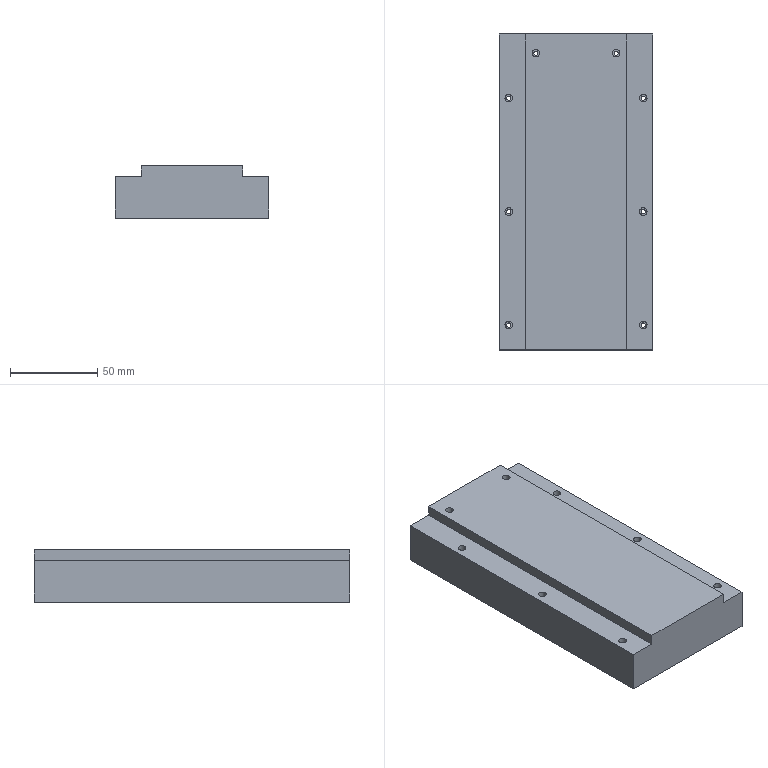NC program | NX | posted with a generic post | part box 88 x 181.05 x 30 mm
Lines 1 to 835 of 7800:
N10 G17 G21 G94 G90
(DYNAMIC_ROUGH_3 , TOOL : D12-36-D12-75-3T-ROUGH)
N12 T02 M6
N14 G54
N16 G17 G0 G90 X-53.494 Y-90.865 B0. C0. S6500 M3
N18 G43 Z44.5 H2
N20 Z2.5
N22 G94 G1 X-53.469 Y-90.864 Z2.344 F3000.
N24 X-53.444 Y-90.863 Z2.282
N26 X-53.419 Y-90.862 Z2.237
N28 X-53.394 Z2.2
N30 X-53.369 Y-90.861 Z2.169
N32 X-53.344 Y-90.86 Z2.143
N34 X-53.319 Y-90.859 Z2.12
N36 X-53.294 Y-90.858 Z2.1
N38 X-53.269 Y-90.857 Z2.082
N40 X-53.244 Z2.067
N42 X-53.219 Y-90.856 Z2.053
N44 X-53.194 Y-90.855 Z2.042
N46 X-53.169 Y-90.854 Z2.032
N48 X-53.144 Y-90.853 Z2.023
N50 X-53.119 Z2.016
N52 X-53.094 Y-90.852 Z2.01
N54 X-53.069 Y-90.851 Z2.006
N56 X-53.044 Y-90.85 Z2.003
N58 X-53.019 Y-90.849 Z2.001
N60 X-52.994 Y-90.848 Z2.
N62 X-51.071 Y-90.786
N64 G3 X-49.994 Y-90.044 R1.213
N66 X-49.296 Y-86.742 R11.454
N68 X-49.012 Y-78.369 R101.327
N70 G1 X-48.991 Y-66.702
N72 X-48.992 Y87.268
N74 G2 X-47.583 Y91.085 R6.181
N76 X-42.354 Y95.358 R9.042
N78 X-40.599 Y95.599 R6.959
N80 G1 X40.825 Y95.593
N82 G2 X44.024 Y94.651 R7.136
N84 X45.858 Y93.313 R8.6
N86 G1 X46.797 Y92.29
N88 X47.561 Y91.162
N90 G2 X48.524 Y87.914 R8.715
N92 X48.938 Y80.429 R68.117
N94 X48.989 Y65.729 R897.026
N96 G1 Y-87.272
N98 G2 X48.498 Y-89.606 R6.42
N100 G1 X48.388 Y-90.627
N102 G2 X47.613 Y-92.691 R7.415
N104 X46.181 Y-94.366 R7.415
N106 X44.264 Y-95.455 R7.415
N108 X42.092 Y-95.825 R7.42
N110 G1 X-42.093
N112 G2 X-44.267 Y-95.454 R7.418
N114 X-46.183 Y-94.365 R7.415
N116 X-47.614 Y-92.688 R7.415
N118 X-48.388 Y-90.625 R7.415
N120 G1 X-48.497 Y-89.525
N122 X-48.496 Y87.668
N124 G2 X-47.809 Y90.683 R7.763
N126 G1 X-47.552 Y91.141
N128 G3 X-47.564 Y92.337 R1.201
N130 G1 X-47.76 Y92.601 Z2.014
N132 X-47.974 Y92.851 Z2.028
N134 X-49.075 Y94.155 Z2.1
N136 X-49.246 Y94.357 F15000.
N138 X-49.408 Y94.568
N140 G2 X-48.929 Y96.28 R1.2
N142 G1 X-45.973 Y97.758
N144 G2 X-39.713 Y99.241 R14.05
N146 G1 X36.838 Y99.361
N148 G2 X37.828 Y98.841 R1.201
N150 G1 X38.015 Y98.57
N152 X39.355 Y96.622 Z2. F3000.
N154 X39.569 Y96.304
N156 X39.797 Y95.995
N158 G3 X40.6 Y95.599 R1.203
N160 G2 X43.374 Y94.98 R7.156
N162 X44.646 Y94.271 R10.832
N164 X45.858 Y93.313 R7.585
N166 G1 X46.797 Y92.29
N168 X47.561 Y91.162
N170 G2 X48.379 Y88.878 R8.612
N172 G1 X48.497 Y87.667
N174 X48.496 Y-89.526
N176 X48.474 Y-89.75
N178 G3 X49.285 Y-91.015 R1.212
N180 G1 X51.167 Y-91.665
N182 X51.19 Y-91.673 Z2.001
N184 X51.214 Y-91.681 Z2.003
N186 X51.238 Y-91.689 Z2.006
N188 X51.261 Y-91.697 Z2.01
N190 X51.285 Y-91.705 Z2.016
N192 X51.308 Y-91.714 Z2.023
N194 X51.332 Y-91.722 Z2.032
N196 X51.356 Y-91.73 Z2.042
N198 X51.379 Y-91.738 Z2.053
N200 X51.403 Y-91.746 Z2.067
N202 X51.427 Y-91.754 Z2.082
N204 X51.45 Y-91.763 Z2.1
N206 X51.474 Y-91.771 Z2.12
N208 X51.497 Y-91.779 Z2.143
N210 X51.521 Y-91.787 Z2.169
N212 X51.545 Y-91.795 Z2.2
N214 X51.568 Y-91.803 Z2.237
N216 X51.592 Y-91.812 Z2.282
N218 X51.616 Y-91.82 Z2.344
N220 X51.639 Y-91.828 Z2.5
N222 G0 Z44.5
N224 X47.588 Y96.389
N226 Z3.3
N228 G1 X47.575 Y96.368 Z3.144
N230 X47.562 Y96.347 Z3.082
N232 X47.549 Y96.325 Z3.037
N234 X47.536 Y96.304 Z3.
N236 X47.522 Y96.283 Z2.969
N238 X47.509 Y96.262 Z2.943
N240 X47.496 Y96.24 Z2.92
N242 X47.483 Y96.219 Z2.9
N244 X47.47 Y96.198 Z2.882
N246 X47.457 Y96.176 Z2.867
N248 X47.444 Y96.155 Z2.853
N250 X47.431 Y96.134 Z2.842
N252 X47.418 Y96.113 Z2.832
N254 X47.405 Y96.091 Z2.823
N256 X47.391 Y96.07 Z2.816
N258 X47.378 Y96.049 Z2.81
N260 X47.365 Y96.027 Z2.806
N262 X47.352 Y96.006 Z2.803
N264 X47.339 Y95.985 Z2.801
N266 X47.326 Y95.963 Z2.8
N268 X46.226 Y94.176
N270 G3 X46.267 Y92.843 R1.212
N272 G2 X47.368 Y90.939 R7.542
N274 X47.776 Y88.71 R7.678
N276 G1 Y-78.044
N278 G3 X47.608 Y-84.969 R114.645
N280 G2 X47.491 Y-87.655 R16.77
N282 X44.801 Y-91.823 R7.045
N284 X39.821 Y-94.05 R12.513
N286 X33.271 Y-94.783 R36.232
N288 X20.897 Y-94.913 R367.986
N290 G1 X-38.887 Y-94.915
N292 G2 X-44.025 Y-92.665 R6.608
N294 X-46.529 Y-87.896 R11.391
N296 X-47.41 Y-81.519 R30.046
N298 G1 X-47.482 Y-80.096
N300 G2 X-47.776 Y-78.057 R7.072
N302 G1 Y88.71
N304 G2 X-47.367 Y90.94 R7.678
N306 X-46.234 Y92.889 R7.645
N308 G1 X-45.436 Y94.526
N310 G3 X-47.269 Y96.008 R1.212
N312 G1 X-47.289 Y95.993 Z2.801
N314 X-47.309 Y95.977 Z2.803
N316 X-47.329 Y95.962 Z2.806
N318 X-47.349 Y95.947 Z2.81
N320 X-47.368 Y95.932 Z2.816
N322 X-47.388 Y95.916 Z2.823
N324 X-47.408 Y95.901 Z2.832
N326 X-47.428 Y95.886 Z2.842
N328 X-47.448 Y95.871 Z2.853
N330 X-47.468 Y95.856 Z2.867
N332 X-47.487 Y95.84 Z2.882
N334 X-47.507 Y95.825 Z2.9
N336 X-47.527 Y95.81 Z2.92
N338 X-47.547 Y95.795 Z2.943
N340 X-47.567 Y95.779 Z2.969
N342 X-47.587 Y95.764 Z3.
N344 X-47.606 Y95.749 Z3.037
N346 X-47.626 Y95.734 Z3.082
N348 X-47.646 Y95.718 Z3.144
N350 X-47.666 Y95.703 Z3.3
N352 G0 Z44.5
N354 X51.149 Y-77.61
N356 Z3.3
N358 G1 X51.128 Y-77.624 Z3.144
N360 X51.107 Y-77.638 Z3.082
N362 X51.086 Y-77.651 Z3.037
N364 X51.066 Y-77.665 Z3.
N366 X51.045 Y-77.679 Z2.969
N368 X51.024 Y-77.693 Z2.943
N370 X51.003 Y-77.707 Z2.92
N372 X50.982 Y-77.72 Z2.9
N374 X50.961 Y-77.734 Z2.882
N376 X50.94 Y-77.748 Z2.867
N378 X50.92 Y-77.762 Z2.853
N380 X50.899 Y-77.776 Z2.842
N382 X50.878 Y-77.789 Z2.832
N384 X50.857 Y-77.803 Z2.823
N386 X50.836 Y-77.817 Z2.816
N388 X50.815 Y-77.831 Z2.81
N390 X50.795 Y-77.845 Z2.806
N392 X50.774 Y-77.858 Z2.803
N394 X50.753 Y-77.872 Z2.801
N396 X50.732 Y-77.886 Z2.8
N398 G2 X50.203 Y-78.079 R1.234
N400 G1 X48.745 Y-78.249
N402 G3 X47.707 Y-79.167 R1.212
N404 X47.105 Y-81.702 R44.542
N406 X46.757 Y-84.555 R170.613
N408 G2 X42.697 Y-90.703 R9.334
N410 X36.882 Y-93.031 R15.758
N412 X29.654 Y-93.776 R44.68
N414 X16.755 Y-93.912 R397.795
N416 G1 X-36.033 Y-93.914
N418 G2 X-42.957 Y-90.434 R8.801
N420 X-45.547 Y-84.787 R14.409
N422 G3 X-45.996 Y-82.71 R53.636
N424 X-46.403 Y-82.153 R1.757
N426 G2 X-47.485 Y-80.086 R6.908
N428 G3 X-46.403 Y-82.153 R6.908
N430 G2 X-45.662 Y-83.309 R2.716
N432 G3 X-44.096 Y-87.04 R47.633
N434 X-40.443 Y-91.177 R9.959
N436 X-35.352 Y-92.872 R13.508
N438 X-28.769 Y-93.276 R51.87
N440 X-18.644 Y-93.314 R719.838
N442 G1 X16.156 Y-93.312
N444 G3 X29.804 Y-93.145 R338.101
N446 X36.865 Y-92.28 R37.702
N448 X42.016 Y-89.937 R13.406
N450 X45.195 Y-85.465 R10.315
N452 X46.186 Y-82.471 R61.029
N454 G1 X46.343 Y-82.217
N456 G2 X47.194 Y-81.825 R1.202
N458 G1 X47.651 Y-81.81
N460 X50.015 Y-81.736 Z2.9
N462 X50.315 Y-81.725 F15000.
N464 X50.615 Y-81.729
N466 G2 X51.483 Y-83.594 R1.2
N468 G1 X51.302 Y-83.865
N470 X51.108 Y-84.128
N472 G2 X49.036 Y-83.545 R1.2
N474 X49.113 Y-82.839 Z2.87 R1.32 F3000.
N476 G1 X49.627 Y-81.276 Z2.8
N478 G3 X49.742 Y-80.598 R1.544
N480 X47.448 Y-80.234 R1.2
N482 G2 X46.401 Y-82.155 R7.336
N484 G3 X45.381 Y-83.538 R6.207
N486 G2 X43.055 Y-86.875 R18.551
N488 X36.847 Y-90.698 R14.372
N490 X29.777 Y-91.976 R30.792
N492 X19.059 Y-92.297 R150.392
N494 G1 X8.634 Y-92.313
N496 X-21.216 Y-92.312
N498 G2 X-31.264 Y-92.158 R199.606
N500 X-36.29 Y-91.371 R20.815
N502 X-41.797 Y-87.349 R11.259
N504 X-43.873 Y-84.193 R39.119
N506 G3 X-44.763 Y-83.601 R2.273
N508 G1 X-45.647 Y-82.948
N510 X-46.112 Y-82.459
N512 G3 X-44.064 Y-83.952 R5.862
N514 G2 X-42.792 Y-85.273 R9.294
N516 G3 X-39.69 Y-88.418 R19.651
N518 X-33.639 Y-90.998 R14.487
N520 X-26.701 Y-91.634 R41.915
N522 X-14.627 Y-91.713 R570.626
N524 G1 X13.123 Y-91.711
N526 G3 X26.546 Y-91.54 R343.845
N528 X34.136 Y-90.665 R43.737
N530 X40.417 Y-87.928 R16.378
N532 X43.773 Y-84.474 R17.766
N534 G2 X44.455 Y-83.754 R2.419
N536 G3 X46.11 Y-82.461 R5.554
N538 G2 X44.052 Y-83.955 R5.829
N540 G3 X41.669 Y-85.699 R35.059
N542 G2 X32.303 Y-89.724 R22.148
N544 X23.578 Y-90.57 R56.766
N546 X8.279 Y-90.711 R501.856
N548 G1 X-15.346 Y-90.712
N550 G2 X-27.419 Y-90.569 R288.361
N552 X-33.577 Y-89.743 R29.409
N554 X-39.78 Y-86.365 R15.598
N556 G3 X-41.853 Y-84.606 R39.593
N558 X-42.728 Y-84.402 R1.968
N560 G1 X-43.781 Y-84.09
N562 X-44.184 Y-83.89
N564 G3 X-42.051 Y-84.482 R5.606
N566 G2 X-40.214 Y-85.511 R8.071
N568 G3 X-35.654 Y-88.13 R25.306
N570 X-28.664 Y-89.752 R24.206
N572 X-19.599 Y-90.094 R102.656
N574 G1 X-11.274 Y-90.112
N576 X9.201 Y-90.11
N578 G3 X24.124 Y-89.927 R379.325
N580 X32.386 Y-88.991 R49.502
N582 X41.184 Y-85.125 R23.99
N584 G2 X42.275 Y-84.472 R5.432
N586 G3 X43.778 Y-84.091 R7.76
N588 G1 X44.114 Y-83.924
N590 G2 X42.048 Y-84.479 R5.545
N592 G3 X39.554 Y-85.359 R14.319
N594 G2 X26.642 Y-88.651 R38.799
N596 X15.553 Y-89.079 R138.342
N598 G1 X3.328 Y-89.111
N600 X-13.697 Y-89.11
N602 G2 X-25.394 Y-88.929 R237.118
N604 X-32.429 Y-87.892 R32.419
N606 X-37.734 Y-85.623 R24.937
N608 G3 X-39.817 Y-84.567 R17.087
N610 G1 X-40.062 Y-84.526
N612 X-41.637
N614 X-42.158 Y-84.467
N616 X-41.637 Y-84.526
N618 X-39.837 Y-84.527
N620 G2 X-37.442 Y-85.316 R10.717
N622 G3 X-30.782 Y-87.53 R34.785
N624 X-22.363 Y-88.398 R49.354
N626 X-8.489 Y-88.511 R485.88
N628 G1 X7.111 Y-88.509
N630 G3 X21.884 Y-88.327 R397.195
N632 X31.27 Y-87.314 R59.307
N634 X38.639 Y-85.035 R44.926
N636 G2 X40.167 Y-84.529 R9.609
N638 G3 X42.082 Y-84.475 R13.976
N640 G2 X40.216 Y-84.526 R12.797
N642 G3 X37.174 Y-84.888 R10.92
N644 G2 X30.25 Y-86.404 R111.025
N646 X19.051 Y-87.375 R81.729
N648 X-0.073 Y-87.51 R737.621
N650 G1 X-11.698 Y-87.508
N652 G2 X-23.694 Y-87.296 R225.827
N654 X-35.583 Y-84.856 R38.078
N656 G3 X-36.694 Y-84.526 R5.346
N658 G1 X-39.919
N660 X-36.187 Y-84.54
N662 G2 X-32.6 Y-85.284 R30.96
N664 G3 X-21.165 Y-86.764 R55.346
N666 X-8.266 Y-86.908 R382.562
N668 G1 X1.934 Y-86.909
N670 G3 X19.332 Y-86.75 R569.007
N672 X31.261 Y-85.552 R76.778
N674 G1 X36.128 Y-84.526
N676 X39.428
N678 G3 X33.248 Y-84.544 R319.2
N680 X26.692 Y-85.219 R271.928
N682 G2 X12.086 Y-85.866 R165.03
N684 X-2.314 Y-85.909 R932.939
N686 G1 X-30.412
N688 G3 X-30.98 Y-86.052 R1.218
N690 X-31.617 Y-87.07 Z2.853 R1.243
N692 G1 X-31.754 Y-88.171 Z2.9
N694 X-32.056 Y-90.58 F15000.
N696 G2 X-34.175 Y-89.671 R-1.2
N698 G1 X-33.901 Y-89.341
N700 X-33.639 Y-89.
N702 G3 X-33.837 Y-87.502 R1.2
N704 X-34.621 Y-87.168 Z2.863 R1.283 F3000.
N706 G1 X-36.104 Y-86.974 Z2.8
N708 X-36.409 Y-86.936
N710 X-36.711 Y-86.883
N712 G2 X-36.394 Y-84.526 R1.2
N714 X-32.159 Y-84.884 R19.712
N716 G3 X-25.499 Y-85.273 R53.938
N718 X-14.25 Y-85.309 R779.238
N720 G1 X27.589
N722 G2 X28.018 Y-85.388 R1.28
N724 G1 X30.363 Y-86.286
N726 X31.675 Y-86.793 Z2.86
N728 G2 X32.308 Y-87.477 Z2.9 R1.2
N730 X31.351 Y-89.071 R1.2 F15000.
N732 G1 X31.052 Y-89.116
N734 X30.751 Y-89.146
N736 G2 X29.632 Y-87.501 R1.2
N738 X30.824 Y-86.749 Z2.836 R1.207 F3000.
N740 G1 X31.68 Y-86.804 Z2.8
N742 X33.5 Y-86.923
N744 G3 X33.578 Y-84.526 R-1.2
N746 G1 X-35.122
N748 G3 X-36.322 Y-85.569 R1.212
N750 G1 X-36.592 Y-87.482
N752 X-36.595 Y-87.506 Z2.801
N754 X-36.599 Y-87.531 Z2.803
N756 X-36.602 Y-87.556 Z2.806
N758 X-36.606 Y-87.581 Z2.81
N760 X-36.609 Y-87.605 Z2.816
N762 X-36.613 Y-87.63 Z2.823
N764 X-36.616 Y-87.655 Z2.832
N766 X-36.62 Y-87.68 Z2.842
N768 X-36.623 Y-87.705 Z2.853
N770 X-36.627 Y-87.729 Z2.867
N772 X-36.63 Y-87.754 Z2.882
N774 X-36.634 Y-87.779 Z2.9
N776 X-36.637 Y-87.804 Z2.92
N778 X-36.641 Y-87.828 Z2.943
N780 X-36.644 Y-87.853 Z2.969
N782 X-36.648 Y-87.878 Z3.
N784 X-36.651 Y-87.903 Z3.037
N786 X-36.655 Y-87.927 Z3.082
N788 X-36.658 Y-87.952 Z3.144
N790 X-36.662 Y-87.977 Z3.3
N792 G0 Z44.5
N794 X-20.835 Y-60.192
N796 Z4.5
N798 G1 X-20.859 Y-60.199 Z4.344
N800 X-20.883 Y-60.207 Z4.282
N802 X-20.907 Y-60.214 Z4.237
N804 X-20.931 Y-60.222 Z4.2
N806 X-20.955 Y-60.229 Z4.169
N808 X-20.979 Y-60.236 Z4.143
N810 X-21.003 Y-60.244 Z4.12
N812 X-21.026 Y-60.251 Z4.1
N814 X-21.05 Y-60.258 Z4.082
N816 X-21.074 Y-60.266 Z4.067
N818 X-21.098 Y-60.273 Z4.053
N820 X-21.122 Y-60.28 Z4.042
N822 X-21.146 Y-60.288 Z4.032
N824 X-21.17 Y-60.295 Z4.023
N826 X-21.194 Y-60.303 Z4.016
N828 X-21.218 Y-60.31 Z4.01
N830 X-21.241 Y-60.317 Z4.006
N832 X-21.265 Y-60.325 Z4.003
N834 X-21.289 Y-60.332 Z4.001
N836 X-21.313 Y-60.339 Z4.
N838 X-23.741 Y-61.088
N840 G3 X-24.402 Y-62.904 R1.212
N842 X-23.645 Y-63.448 R1.37
N844 X-20.583 Y-64.032 R12.511
N846 G1 X22.575 Y-64.018
N848 G3 X24.386 Y-63.32 R3.079
N850 X24.684 Y-62.806 R1.494
N852 X23.101 Y-61.185 R1.32
N854 G1 X22.084 Y-61.429
N856 G3 X22.392 Y-64.032 R1.32
N858 X23.631 Y-63.98 R5.91
N860 X24.783 Y-62.672 R1.384
N862 X22.068 Y-62.078 R1.436
N864 X23.292 Y-64.032 R1.36
N866 X24.769 Y-62.485 R1.32
N868 X24.08 Y-61.559 R1.201
N870 G1 X23.456 Y-61.273
N872 X21.305 Y-60.289 Z4.1
N874 G3 X20.737 Y-60.158 R1.239 F15000.
N876 G1 X-17.291 Y-60.741
N878 G3 X-18.09 Y-61.061 R1.203
N880 X-18.421 Y-61.525 Z4.076 R1.886 F3000.
N882 G1 X-19.33 Y-63.069 Z4.
N884 X-19.478 Y-63.323
N886 X-19.637 Y-63.57
N888 G2 X-20.583 Y-64.032 R1.201
N890 X-22.677 Y-63.972 R15.085
N892 X-24.453 Y-63.124 R2.882
N894 G1 X-24.607 Y-62.867
N896 G2 X-23.139 Y-61.186 R1.223
N898 G1 X-21.651 Y-61.641
N900 G2 X-22.008 Y-64.032 R1.223
N902 X-23.49 Y-63.908 R4.537
N904 X-24.677 Y-62.916 R1.744
N906 G1 X-24.718 Y-62.772
N908 G2 X-22.999 Y-61.262 R1.32
N910 G1 X-22.62 Y-61.389
N912 X-22.246 Y-61.53
N914 G2 X-22.833 Y-64.032 R1.32
N916 X-24.55 Y-63.347 R1.912
N918 X-24.774 Y-62.643 R1.368
N920 X-22.976 Y-61.464 R1.275
N922 G1 X-22.752 Y-61.565
N924 X-22.532 Y-61.676
N926 G2 X-23.208 Y-64.032 R1.275
N928 X-24.729 Y-63.118 R1.415
N930 X-24.769 Y-62.485 R1.46
N932 G3 X-24.774 Y-62.929 R1.283
N934 X-23.545 Y-64.029 R1.269
N936 X-22.39 Y-63.354 R1.212
N938 G1 X-21.266 Y-61.069
N940 X-21.255 Y-61.046 Z4.001
N942 X-21.244 Y-61.024 Z4.003
N944 X-21.233 Y-61.002 Z4.006
N946 X-21.221 Y-60.979 Z4.01
N948 X-21.21 Y-60.957 Z4.016
N950 X-21.199 Y-60.934 Z4.023
N952 X-21.188 Y-60.912 Z4.032
N954 X-21.177 Y-60.889 Z4.042
N956 X-21.166 Y-60.867 Z4.053
N958 X-21.155 Y-60.845 Z4.067
N960 X-21.144 Y-60.822 Z4.082
N962 X-21.133 Y-60.8 Z4.1
N964 X-21.122 Y-60.777 Z4.12
N966 X-21.111 Y-60.755 Z4.143
N968 X-21.1 Y-60.732 Z4.169
N970 X-21.089 Y-60.71 Z4.2
N972 X-21.078 Y-60.688 Z4.237
N974 X-21.067 Y-60.665 Z4.282
N976 X-21.056 Y-60.643 Z4.344
N978 X-21.045 Y-60.62 Z4.5
N980 G0 Z44.5
N982 X-51.291 Y-78.418
N984 Z3.5
N986 G1 X-51.266 Y-78.417 Z3.344
N988 X-51.241 Y-78.416 Z3.282
N990 X-51.216 Y-78.415 Z3.237
N992 X-51.191 Y-78.414 Z3.2
N994 X-51.166 Y-78.412 Z3.169
N996 X-51.141 Y-78.411 Z3.143
N998 X-51.116 Y-78.41 Z3.12
N1000 X-51.091 Y-78.409 Z3.1
N1002 X-51.066 Y-78.408 Z3.082
N1004 X-51.041 Y-78.407 Z3.067
N1006 X-51.016 Y-78.405 Z3.053
N1008 X-50.991 Y-78.404 Z3.042
N1010 X-50.966 Y-78.403 Z3.032
N1012 X-50.941 Y-78.402 Z3.023
N1014 X-50.916 Y-78.401 Z3.016
N1016 X-50.891 Y-78.399 Z3.01
N1018 X-50.866 Y-78.398 Z3.006
N1020 X-50.841 Y-78.397 Z3.003
N1022 X-50.816 Y-78.396 Z3.001
N1024 X-50.791 Y-78.395 Z3.
N1026 X-48.838 Y-78.302
N1028 G3 X-47.79 Y-77.591 R1.213
N1030 X-47.603 Y-76.969 R2.105
N1032 G1 Y88.891
N1034 G2 X-47.208 Y91.075 R7.266
N1036 X-46.074 Y92.982 R7.263
N1038 X-44.344 Y94.371 R7.263
N1040 X-41.314 Y95.157 R7.193
N1042 G1 X41.314 Y95.156
N1044 G2 X43.467 Y94.775 R7.323
N1046 X45.358 Y93.681 R7.32
N1048 X46.762 Y92.006 R7.32
N1050 X47.508 Y89.952 R7.32
N1052 G1 X47.603 Y88.86
N1054 Y-77.201
N1056 G2 X47.275 Y-79.392 R7.387
N1058 X46.228 Y-81.312 R7.336
N1060 X44.588 Y-82.759 R7.336
N1062 X42.552 Y-83.559 R7.336
N1064 X39.283 Y-83.649 R15.108
N1066 G1 X37.594 Y-83.603
N1068 G2 X36.758 Y-83.684 R13.426
N1070 G1 X-36.872 Y-83.685
N1072 X-39.243 Y-83.58
N1074 G2 X-42.555 Y-83.559 R11.029
N1076 X-44.59 Y-82.758 R7.336
N1078 X-46.23 Y-81.31 R7.336
N1080 X-47.276 Y-79.389 R7.336
N1082 X-47.603 Y-77.214 R7.333
N1084 G1 Y-76.914
N1086 X-47.534 Y-78.322
N1088 G3 X-46.837 Y-80.395 R7.336
N1090 X-45.473 Y-82.106 R7.336
N1092 X-43.607 Y-83.247 R7.336
N1094 X-41.462 Y-83.683 R7.337
N1096 X-38.985 Y-83.558 R13.049
N1098 G2 X-36.872 Y-83.685 R10.37
N1100 X-36.002 Y-84.229 R1.202
N1102 G1 X-35.721 Y-84.667
N1104 X-34.551 Y-86.481 Z3.091
N1106 X-34.418 Y-86.638 Z3.1
N1108 G3 X-33.58 Y-86.977 R1.203 F15000.
N1110 G1 X34.302 Y-86.894
N1112 G3 X35.017 Y-86.657 R1.207
N1114 X35.371 Y-86.249 Z3.077 R1.414 F3000.
N1116 G1 X36.358 Y-84.72 Z3.
N1118 X36.583 Y-84.367
N1120 X36.819 Y-84.022
N1122 G2 X37.594 Y-83.603 R1.203
N1124 X40.146 Y-83.687 R9.14
N1126 X41.177 Y-84.591 R1.212
N1128 G1 X41.696 Y-86.626
N1130 X41.702 Y-86.65 Z3.001
N1132 X41.709 Y-86.674 Z3.003
N1134 X41.715 Y-86.699 Z3.006
N1136 X41.721 Y-86.723 Z3.01
N1138 X41.727 Y-86.747 Z3.016
N1140 X41.733 Y-86.771 Z3.023
N1142 X41.74 Y-86.795 Z3.032
N1144 X41.746 Y-86.82 Z3.042
N1146 X41.752 Y-86.844 Z3.053
N1148 X41.758 Y-86.868 Z3.067
N1150 X41.764 Y-86.892 Z3.082
N1152 X41.77 Y-86.917 Z3.1
N1154 X41.777 Y-86.941 Z3.12
N1156 X41.783 Y-86.965 Z3.143
N1158 X41.789 Y-86.989 Z3.169
N1160 X41.795 Y-87.013 Z3.2
N1162 X41.801 Y-87.038 Z3.237
N1164 X41.808 Y-87.062 Z3.282
N1166 X41.814 Y-87.086 Z3.344
N1168 X41.82 Y-87.11 Z3.5
N1170 G0 Z44.5
N1172 X-51.118 Y-74.04
N1174 Z4.5
N1176 G1 X-51.093 Y-74.039 Z4.344
N1178 X-51.068 Y-74.037 Z4.282
N1180 X-51.043 Y-74.036 Z4.237
N1182 X-51.018 Y-74.035 Z4.2
N1184 X-50.993 Y-74.033 Z4.169
N1186 X-50.968 Y-74.032 Z4.143
N1188 X-50.943 Y-74.03 Z4.12
N1190 X-50.918 Y-74.029 Z4.1
N1192 X-50.893 Y-74.028 Z4.082
N1194 X-50.868 Y-74.026 Z4.067
N1196 X-50.843 Y-74.025 Z4.053
N1198 X-50.818 Y-74.024 Z4.042
N1200 X-50.793 Y-74.022 Z4.032
N1202 X-50.768 Y-74.021 Z4.023
N1204 X-50.743 Y-74.019 Z4.016
N1206 X-50.718 Y-74.018 Z4.01
N1208 X-50.693 Y-74.017 Z4.006
N1210 X-50.668 Y-74.015 Z4.003
N1212 X-50.643 Y-74.014 Z4.001
N1214 X-50.618 Y-74.012 Z4.
N1216 X-48.647 Y-73.903
N1218 G3 X-47.618 Y-73.208 R1.213
N1220 X-46.965 Y-70.419 R9.276
N1222 X-46.703 Y-66.317 R55.536
N1224 G1 X-46.705 Y-12.068
N1226 G3 X-46.703 Y-10.26 R10.908
N1228 G1 X-46.702 Y88.454
N1230 G2 X-46.315 Y90.594 R7.288
N1232 X-45.22 Y92.473 R7.285
N1234 X-43.548 Y93.864 R7.285
N1236 X-41.501 Y94.6 R7.285
N1238 G1 X-40.412 Y94.69
N1240 X40.412
N1242 G2 X42.559 Y94.321 R7.292
N1244 X44.447 Y93.24 R7.285
N1246 X45.851 Y91.58 R7.285
N1248 X46.603 Y89.539 R7.285
N1250 G1 X46.702 Y88.452
N1252 X46.704 Y-10.264
N1254 G3 X46.703 Y-12.19 R13.522
N1256 G1 X46.702 Y-72.823
N1258 G2 X46.598 Y-75.106 R96.553
N1260 X44.071 Y-79.364 R6.634
N1262 X38.504 Y-81.87 R13.216
N1264 X32.023 Y-82.557 R37.881
N1266 X19.874 Y-82.681 R380.762
N1268 G1 X-33.226 Y-82.683
N1270 G3 X-38.571 Y-82.631 R165.405
N1272 G2 X-42.877 Y-80.578 R6.484
N1274 X-44.817 Y-77.518 R9.165
N1276 G3 X-45.329 Y-76.932 R4.428
N1278 G2 X-46.376 Y-75.011 R7.336
N1280 X-46.703 Y-72.836 R7.333
N1282 G1 Y-66.311
N1284 Y-72.836
N1286 G3 X-46.376 Y-75.011 R7.36
N1288 X-45.329 Y-76.932 R7.336
N1290 G1 X-43.63 Y-78.767
N1292 G3 X-39.044 Y-81.185 R10.444
N1294 X-32.883 Y-81.975 R28.137
N1296 X-19.834 Y-82.082 R404.652
N1298 G1 X19.991 Y-82.08
N1300 G3 X32.289 Y-81.917 R283.811
N1302 X38.375 Y-81.11 R29.959
N1304 X41.791 Y-79.618 R10.146
N1306 G1 X42.722 Y-78.862
N1308 G3 X44.571 Y-77.729 R7.249
N1310 X45.935 Y-76.02 R7.336
N1312 X46.633 Y-73.947 R7.336
N1314 G1 X46.67 Y-73.348
N1316 X46.633 Y-73.947
N1318 G2 X45.935 Y-76.02 R7.336
N1320 X44.571 Y-77.729 R7.336
N1322 X42.705 Y-78.87 R7.336
N1324 X30.846 Y-80.878 R45.188
N1326 X18.699 Y-81.075 R276.781
N1328 G1 X10.449 Y-81.082
N1330 X-35.751 Y-81.077
N1332 G2 X-40.16 Y-79.378 R18.014
N1334 G3 X-41.654 Y-79.181 R10.771
N1336 G2 X-43.69 Y-78.38 R7.336
N1338 G1 X-44.573 Y-77.728
N1340 X-44.779 Y-77.51
N1342 X-44.573 Y-77.728
N1344 G3 X-42.707 Y-78.869 R7.336
N1346 X-40.289 Y-79.307 R7.174
N1348 G1 X-37.72 Y-79.899
N1350 G3 X-31.374 Y-80.423 R39.225
N1352 X-18.924 Y-80.481 R760.897
N1354 G1 X34.571 Y-80.476
N1356 G3 X36.242 Y-79.985 R53.443
N1358 G2 X38.923 Y-79.305 R37.111
N1360 G1 X40.561
N1362 X41.652 Y-79.181
N1364 X40.561 Y-79.305
N1366 G3 X34.568 Y-79.403 R105.956
N1368 G2 X18.518 Y-79.481 R867.565
N1370 G1 X-34.38 Y-79.476
N1372 X-35.365 Y-79.305
N1374 X-40.39
N1376 X37.31
N1378 G2 X38.521 Y-80.557 R1.212
N1380 G1 X38.465 Y-82.261
N1382 X38.464 Y-82.286 Z4.001
N1384 X38.463 Y-82.311 Z4.003
N1386 Y-82.336 Z4.006
N1388 X38.462 Y-82.361 Z4.01
N1390 X38.461 Y-82.386 Z4.016
N1392 X38.46 Y-82.411 Z4.023
N1394 X38.459 Y-82.436 Z4.032
N1396 X38.458 Y-82.461 Z4.042
N1398 Y-82.486 Z4.053
N1400 X38.457 Y-82.511 Z4.067
N1402 X38.456 Y-82.536 Z4.082
N1404 X38.455 Y-82.561 Z4.1
N1406 X38.454 Y-82.586 Z4.12
N1408 X38.453 Y-82.611 Z4.143
N1410 Y-82.636 Z4.169
N1412 X38.452 Y-82.661 Z4.2
N1414 X38.451 Y-82.686 Z4.237
N1416 X38.45 Y-82.711 Z4.282
N1418 X38.449 Y-82.736 Z4.344
N1420 X38.448 Y-82.761 Z4.5
N1422 G0 Z44.5
N1424 X-20.957 Y-60.676
N1426 Z5.5
N1428 G1 X-20.98 Y-60.686 Z5.344
N1430 X-21.004 Y-60.695 Z5.282
N1432 X-21.027 Y-60.704 Z5.237
N1434 X-21.05 Y-60.714 Z5.2
N1436 X-21.073 Y-60.723 Z5.169
N1438 X-21.096 Y-60.732 Z5.143
N1440 X-21.119 Y-60.742 Z5.12
N1442 X-21.143 Y-60.751 Z5.1
N1444 X-21.166 Y-60.76 Z5.082
N1446 X-21.189 Y-60.77 Z5.067
N1448 X-21.212 Y-60.779 Z5.053
N1450 X-21.235 Y-60.788 Z5.042
N1452 X-21.259 Y-60.798 Z5.032
N1454 X-21.282 Y-60.807 Z5.023
N1456 X-21.305 Y-60.816 Z5.016
N1458 X-21.328 Y-60.826 Z5.01
N1460 X-21.351 Y-60.835 Z5.006
N1462 X-21.375 Y-60.844 Z5.003
N1464 X-21.398 Y-60.854 Z5.001
N1466 X-21.421 Y-60.863 Z5.
N1468 X-24.109 Y-61.947
N1470 G3 X-24.841 Y-62.818 R1.213
N1472 X-24.028 Y-64.092 R1.192
N1474 X-20.999 Y-64.715 R11.255
N1476 X-12.798 Y-65.01 R96.255
N1478 G1 X-2.481 Y-65.032
N1480 X20.65 Y-65.03
N1482 G3 X23.399 Y-64.707 R8.932
N1484 X24.771 Y-63.639 R2.27
N1486 X24.871 Y-62.979 R1.488
N1488 X23.982 Y-61.988 R1.2
N1490 G1 X23.817 Y-61.946
N1492 X21.527 Y-61.357 Z5.1
N1494 X21.262 Y-61.289 F15000.
N1496 X21. Y-61.211
N1498 G2 X20.263 Y-60.318 R1.201
N1500 X20.293 Y-59.503 R1.368
N1502 X20.982 Y-58.816 R1.202
N1504 X22.386 Y-59.234 Z5.033 R1.205 F3000.
N1506 G1 X22.847 Y-59.874 Z5.
N1508 X24.639 Y-62.359
N1510 G2 X24.841 Y-62.819 R1.244
N1512 X24.526 Y-64.137 R1.284
N1514 X22.663 Y-65.127 R3.556
N1516 X18.649 Y-65.537 R21.637
N1518 X8.727 Y-65.632 R357.877
N1520 G1 X-5.967 Y-65.631
N1522 G2 X-18.303 Y-65.466 R275.89
N1524 X-22.847 Y-64.889 R22.716
N1526 X-24.612 Y-63.901 R3.439
N1528 X-24.871 Y-62.985 R1.315
N1530 X-24.046 Y-61.998 R1.201
N1532 X-23.265 Y-62.01 Z5.034 R1.29
N1534 G1 X-21.747 Y-62.413 Z5.1
N1536 X-21.405 Y-62.507 F15000.
N1538 X-21.058 Y-62.584
N1540 G3 X-19.732 Y-61.608 R1.2
N1542 X-19.714 Y-60.951 R1.454
N1544 X-21.244 Y-60.082 R1.2
N1546 X-21.731 Y-60.348 Z5.076 R1.909 F3000.
N1548 G1 X-23.24 Y-61.343 Z5.
N1550 X-24.326 Y-62.058
N1552 G3 X-24.841 Y-62.818 R1.203
N1554 X-24.48 Y-64.295 R1.39
N1556 X-22.291 Y-65.52 R5.101
N1558 X-17.315 Y-66.345 R22.486
N1560 X-7.188 Y-66.619 R152.907
N1562 G1 X0.594 Y-66.631
N1564 G3 X16.949 Y-66.559 R779.854
N1566 X21.645 Y-66.13 R27.246
N1568 X24.348 Y-64.897 R5.761
N1570 X24.994 Y-63.675 R1.673
N1572 X24.878 Y-63.001 R11.864
N1574 G2 X25.028 Y-63.887 R5.977
N1576 X24.227 Y-65.207 R2.234
N1578 X21.538 Y-66.486 R6.409
N1580 X16.286 Y-67.1 R27.146
N1582 X4.603 Y-67.232 R317.214
N1584 X-13.017 Y-67.129 R745.744
N1586 X-20.053 Y-66.543 R49.012
N1588 X-23.594 Y-65.352 R10.53
N1590 X-24.892 Y-63.99 R3.093
N1592 X-24.895 Y-63.085 R1.498
N1594 G3 X-24.98 Y-64.043 R2.108
N1596 X-23.746 Y-65.673 R3.124
N1598 X-20.271 Y-67.17 R9.77
N1600 X-13.683 Y-68.009 R36.298
N1602 X-0.373 Y-68.226 R280.106
N1604 X14.744 Y-68.122 R503.532
N1606 X20.616 Y-67.515 R32.955
N1608 X23.995 Y-66.074 R8.567
N1610 X25.079 Y-64.74 R3.141
N1612 X25.121 Y-64.183 R1.769
N1614 G1 X24.985 Y-63.522
N1616 X25.167 Y-64.479
N1618 G2 X24.38 Y-65.987 R2.469
N1620 X21.781 Y-67.553 R7.153
N1622 G3 X20.62 Y-69.081 R3.144
N1624 X21.12 Y-73.897 R5.349
N1626 X25.382 Y-77.341 R8.65
N1628 X30.718 Y-78.468 R18.288
N1630 X38.588 Y-78.666 R84.113
N1632 X43.302 Y-76.039 R6.792
N1634 X45.462 Y-71.145 R11.374
N1636 X46.022 Y-65.455 R31.877
N1638 X46.103 Y-52.555 R556.768
N1640 G1 Y-14.737
N1642 X46.102 Y-5.159
N1644 X46.101 Y86.041
N1646 G3 X45.799 Y88.016 R7.154
N1648 X45.416 Y90.126 R7.155
N1650 X44.321 Y92.005 R7.285
N1652 X42.649 Y93.397 R7.285
N1654 X40.602 Y94.133 R7.285
N1656 G1 X39.513 Y94.224
N1658 X-39.512
N1660 G3 X-41.655 Y93.855 R7.289
N1662 X-43.544 Y92.776 R7.285
N1664 X-44.949 Y91.116 R7.285
N1666 X-45.841 Y87.884 R7.26
N1668 X-46.092 Y79.49 R103.706